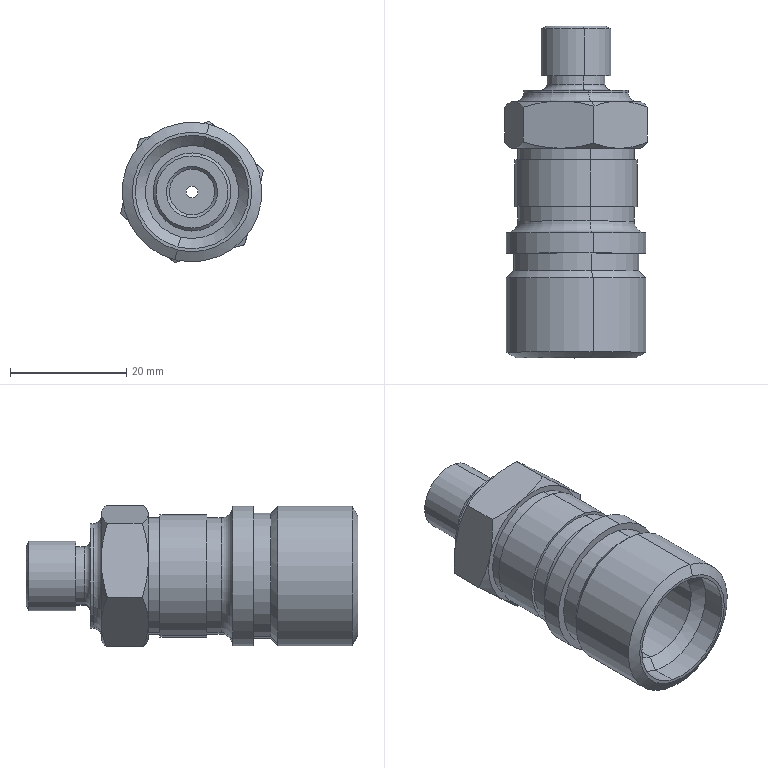Part | SolidWorks | features BaseBody 1 | 1 solid | 79 faces | box 24.547 x 57 x 24.237 mm | volume 14345 mm3 | cone 29 | cylinder 26 | plane 18 | torus 6 | commonest cylinder face diameters 20 x4 24 x4 2 x2 7.8 x2 10 x2 12 x2